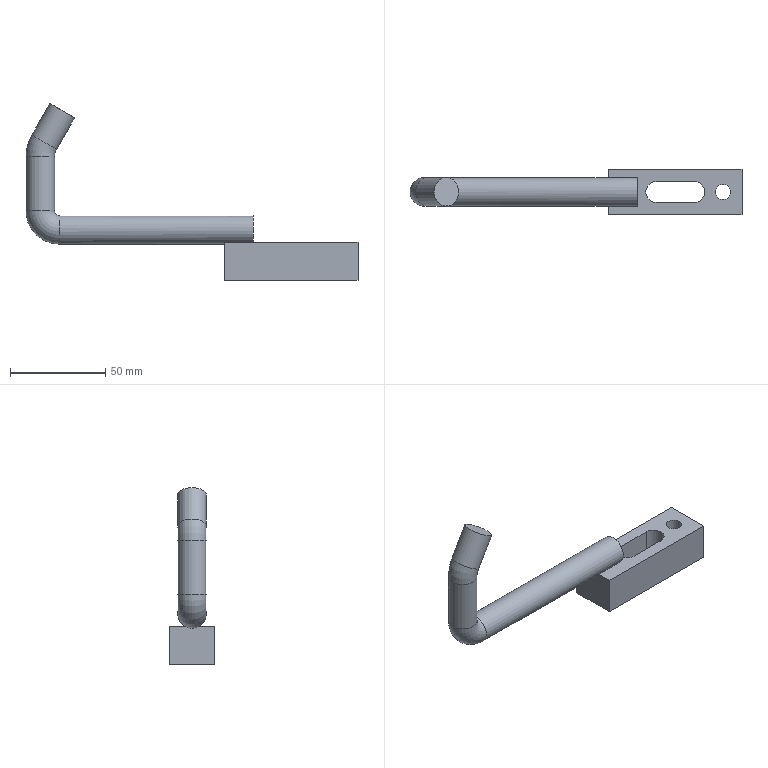Part | NX | features solid 2 | 1 solid | 18 faces | box 174.2 x 24 x 92.75 mm | volume 56758 mm3 | plane 10 | cylinder 6 | torus 2 | commonest cylinder face diameters 15 x3 11 x2 8 x1
STEP:
#1=CARTESIAN_POINT('',(-380.,96.04,-15.));
#2=VERTEX_POINT('',#1);
#3=CARTESIAN_POINT('',(-380.,120.04,-15.));
#4=VERTEX_POINT('',#3);
#5=CARTESIAN_POINT('',(-380.,96.04,-15.));
#6=DIRECTION('',(0.,1.,0.));
#7=VECTOR('',#6,1000.);
#8=LINE('',#5,#7);
#9=EDGE_CURVE('',#2,#4,#8,.T.);
#10=ORIENTED_EDGE('',*,*,#9,.T.);
#11=CARTESIAN_POINT('',(-310.,120.04,-15.));
#12=VERTEX_POINT('',#11);
#13=CARTESIAN_POINT('',(-380.,120.04,-15.));
#14=DIRECTION('',(1.,0.,0.));
#15=VECTOR('',#14,1000.);
#16=LINE('',#13,#15);
#17=EDGE_CURVE('',#4,#12,#16,.T.);
#18=ORIENTED_EDGE('',*,*,#17,.T.);
#19=CARTESIAN_POINT('',(-310.,96.04,-15.));
#20=VERTEX_POINT('',#19);
#21=CARTESIAN_POINT('',(-310.,120.04,-15.));
#22=DIRECTION('',(0.,-1.,0.));
#23=VECTOR('',#22,1000.);
#24=LINE('',#21,#23);
#25=EDGE_CURVE('',#12,#20,#24,.T.);
#26=ORIENTED_EDGE('',*,*,#25,.T.);
#27=CARTESIAN_POINT('',(-310.,96.04,-15.));
#28=DIRECTION('',(-1.,0.,0.));
#29=VECTOR('',#28,1000.);
#30=LINE('',#27,#29);
#31=EDGE_CURVE('',#20,#2,#30,.T.);
#32=ORIENTED_EDGE('',*,*,#31,.T.);
#33=EDGE_LOOP('',(#10,#18,#26,#32));
#34=FACE_BOUND('',#33,.T.);
#35=CARTESIAN_POINT('',(-335.,113.54,-15.));
#36=VERTEX_POINT('',#35);
#37=CARTESIAN_POINT('',(-335.,102.54,-15.));
#38=VERTEX_POINT('',#37);
#39=CARTESIAN_POINT('',(-335.,108.04,-15.));
#40=DIRECTION('',(0.,0.,-1.));
#41=DIRECTION('',(1.,0.,0.));
#42=AXIS2_PLACEMENT_3D('',#39,#40,#41);
#43=CIRCLE('',#42,5.5);
#44=EDGE_CURVE('',#36,#38,#43,.T.);
#45=ORIENTED_EDGE('',*,*,#44,.F.);
#46=CARTESIAN_POINT('',(-355.,113.54,-15.));
#47=VERTEX_POINT('',#46);
#48=CARTESIAN_POINT('',(-355.,113.54,-15.));
#49=DIRECTION('',(1.,0.,0.));
#50=VECTOR('',#49,1000.);
#51=LINE('',#48,#50);
#52=EDGE_CURVE('',#47,#36,#51,.T.);
#53=ORIENTED_EDGE('',*,*,#52,.F.);
#54=CARTESIAN_POINT('',(-355.,102.54,-15.));
#55=VERTEX_POINT('',#54);
#56=CARTESIAN_POINT('',(-355.,108.04,-15.));
#57=DIRECTION('',(0.,0.,-1.));
#58=DIRECTION('',(1.,0.,0.));
#59=AXIS2_PLACEMENT_3D('',#56,#57,#58);
#60=CIRCLE('',#59,5.5);
#61=EDGE_CURVE('',#55,#47,#60,.T.);
#62=ORIENTED_EDGE('',*,*,#61,.F.);
#63=CARTESIAN_POINT('',(-355.,102.54,-15.));
#64=DIRECTION('',(1.,0.,0.));
#65=VECTOR('',#64,1000.);
#66=LINE('',#63,#65);
#67=EDGE_CURVE('',#55,#38,#66,.T.);
#68=ORIENTED_EDGE('',*,*,#67,.T.);
#69=EDGE_LOOP('',(#45,#53,#62,#68));
#70=FACE_BOUND('',#69,.T.);
#71=CARTESIAN_POINT('',(-316.,108.04,-15.));
#72=VERTEX_POINT('',#71);
#73=CARTESIAN_POINT('',(-320.,108.04,-15.));
#74=DIRECTION('',(0.,0.,-1.));
#75=DIRECTION('',(1.,0.,0.));
#76=AXIS2_PLACEMENT_3D('',#73,#74,#75);
#77=CIRCLE('',#76,4.);
#78=EDGE_CURVE('',#72,#72,#77,.T.);
#79=ORIENTED_EDGE('',*,*,#78,.F.);
#80=EDGE_LOOP('',(#79));
#81=FACE_BOUND('',#80,.T.);
#82=CARTESIAN_POINT('',(-310.,96.04,-15.));
#83=DIRECTION('',(0.,0.,1.));
#84=DIRECTION('',(1.,0.,0.));
#85=AXIS2_PLACEMENT_3D('',#82,#83,#84);
#86=PLANE('',#85);
#87=ADVANCED_FACE('',(#34,#70,#81),#86,.F.);
#88=ORIENTED_EDGE('',*,*,#17,.F.);
#89=CARTESIAN_POINT('',(-380.,120.04,5.));
#90=VERTEX_POINT('',#89);
#91=CARTESIAN_POINT('',(-380.,120.04,5.));
#92=DIRECTION('',(0.,0.,-1.));
#93=VECTOR('',#92,1000.);
#94=LINE('',#91,#93);
#95=EDGE_CURVE('',#90,#4,#94,.T.);
#96=ORIENTED_EDGE('',*,*,#95,.F.);
#97=CARTESIAN_POINT('',(-310.,120.04,5.));
#98=VERTEX_POINT('',#97);
#99=CARTESIAN_POINT('',(-380.,120.04,5.));
#100=DIRECTION('',(1.,0.,0.));
#101=VECTOR('',#100,1000.);
#102=LINE('',#99,#101);
#103=EDGE_CURVE('',#90,#98,#102,.T.);
#104=ORIENTED_EDGE('',*,*,#103,.T.);
#105=CARTESIAN_POINT('',(-310.,120.04,5.));
#106=DIRECTION('',(0.,0.,-1.));
#107=VECTOR('',#106,1000.);
#108=LINE('',#105,#107);
#109=EDGE_CURVE('',#98,#12,#108,.T.);
#110=ORIENTED_EDGE('',*,*,#109,.T.);
#111=EDGE_LOOP('',(#88,#96,#104,#110));
#112=FACE_BOUND('',#111,.T.);
#113=CARTESIAN_POINT('',(-380.,120.04,5.));
#114=DIRECTION('',(0.,-1.,0.));
#115=DIRECTION('',(-1.,0.,0.));
#116=AXIS2_PLACEMENT_3D('',#113,#114,#115);
#117=PLANE('',#116);
#118=ADVANCED_FACE('',(#112),#117,.F.);
#119=ORIENTED_EDGE('',*,*,#25,.F.);
#120=ORIENTED_EDGE('',*,*,#109,.F.);
#121=CARTESIAN_POINT('',(-310.,96.04,5.));
#122=VERTEX_POINT('',#121);
#123=CARTESIAN_POINT('',(-310.,120.04,5.));
#124=DIRECTION('',(0.,-1.,0.));
#125=VECTOR('',#124,1000.);
#126=LINE('',#123,#125);
#127=EDGE_CURVE('',#98,#122,#126,.T.);
#128=ORIENTED_EDGE('',*,*,#127,.T.);
#129=CARTESIAN_POINT('',(-310.,96.04,5.));
#130=DIRECTION('',(0.,0.,-1.));
#131=VECTOR('',#130,1000.);
#132=LINE('',#129,#131);
#133=EDGE_CURVE('',#122,#20,#132,.T.);
#134=ORIENTED_EDGE('',*,*,#133,.T.);
#135=EDGE_LOOP('',(#119,#120,#128,#134));
#136=FACE_BOUND('',#135,.T.);
#137=CARTESIAN_POINT('',(-310.,120.04,5.));
#138=DIRECTION('',(-1.,0.,0.));
#139=DIRECTION('',(0.,0.,1.));
#140=AXIS2_PLACEMENT_3D('',#137,#138,#139);
#141=PLANE('',#140);
#142=ADVANCED_FACE('',(#136),#141,.F.);
#143=ORIENTED_EDGE('',*,*,#31,.F.);
#144=ORIENTED_EDGE('',*,*,#133,.F.);
#145=CARTESIAN_POINT('',(-380.,96.04,5.));
#146=VERTEX_POINT('',#145);
#147=CARTESIAN_POINT('',(-310.,96.04,5.));
#148=DIRECTION('',(-1.,0.,0.));
#149=VECTOR('',#148,1000.);
#150=LINE('',#147,#149);
#151=EDGE_CURVE('',#122,#146,#150,.T.);
#152=ORIENTED_EDGE('',*,*,#151,.T.);
#153=CARTESIAN_POINT('',(-380.,96.04,5.));
#154=DIRECTION('',(0.,0.,-1.));
#155=VECTOR('',#154,1000.);
#156=LINE('',#153,#155);
#157=EDGE_CURVE('',#146,#2,#156,.T.);
#158=ORIENTED_EDGE('',*,*,#157,.T.);
#159=EDGE_LOOP('',(#143,#144,#152,#158));
#160=FACE_BOUND('',#159,.T.);
#161=CARTESIAN_POINT('',(-310.,96.04,5.));
#162=DIRECTION('',(0.,1.,0.));
#163=DIRECTION('',(1.,0.,0.));
#164=AXIS2_PLACEMENT_3D('',#161,#162,#163);
#165=PLANE('',#164);
#166=ADVANCED_FACE('',(#160),#165,.F.);
#167=CARTESIAN_POINT('',(-380.,104.298,5.));
#168=VERTEX_POINT('',#167);
#169=CARTESIAN_POINT('',(-380.,96.04,5.));
#170=DIRECTION('',(0.,1.,0.));
#171=VECTOR('',#170,1000.);
#172=LINE('',#169,#171);
#173=EDGE_CURVE('',#146,#168,#172,.T.);
#174=ORIENTED_EDGE('',*,*,#173,.T.);
#175=CARTESIAN_POINT('',(-380.,111.781,5.));
#176=VERTEX_POINT('',#175);
#177=CARTESIAN_POINT('',(-380.,108.04,11.5));
#178=DIRECTION('',(1.,0.,0.));
#179=DIRECTION('',(0.,0.,-1.));
#180=AXIS2_PLACEMENT_3D('',#177,#178,#179);
#181=CIRCLE('',#180,7.5);
#182=EDGE_CURVE('',#168,#176,#181,.T.);
#183=ORIENTED_EDGE('',*,*,#182,.T.);
#184=CARTESIAN_POINT('',(-380.,96.04,5.));
#185=DIRECTION('',(0.,1.,0.));
#186=VECTOR('',#185,1000.);
#187=LINE('',#184,#186);
#188=EDGE_CURVE('',#176,#90,#187,.T.);
#189=ORIENTED_EDGE('',*,*,#188,.T.);
#190=ORIENTED_EDGE('',*,*,#95,.T.);
#191=ORIENTED_EDGE('',*,*,#9,.F.);
#192=ORIENTED_EDGE('',*,*,#157,.F.);
#193=EDGE_LOOP('',(#174,#183,#189,#190,#191,#192));
#194=FACE_BOUND('',#193,.T.);
#195=CARTESIAN_POINT('',(-380.,96.04,5.));
#196=DIRECTION('',(1.,0.,0.));
#197=DIRECTION('',(0.,0.,-1.));
#198=AXIS2_PLACEMENT_3D('',#195,#196,#197);
#199=PLANE('',#198);
#200=ADVANCED_FACE('',(#194),#199,.F.);
#201=CARTESIAN_POINT('',(-335.,113.54,5.));
#202=VERTEX_POINT('',#201);
#203=CARTESIAN_POINT('',(-335.,102.54,5.));
#204=VERTEX_POINT('',#203);
#205=CARTESIAN_POINT('',(-335.,108.04,5.));
#206=DIRECTION('',(0.,0.,-1.));
#207=DIRECTION('',(1.,0.,0.));
#208=AXIS2_PLACEMENT_3D('',#205,#206,#207);
#209=CIRCLE('',#208,5.5);
#210=EDGE_CURVE('',#202,#204,#209,.T.);
#211=ORIENTED_EDGE('',*,*,#210,.F.);
#212=CARTESIAN_POINT('',(-335.,113.54,5.));
#213=DIRECTION('',(0.,0.,1.));
#214=VECTOR('',#213,1000.);
#215=LINE('',#212,#214);
#216=EDGE_CURVE('',#36,#202,#215,.T.);
#217=ORIENTED_EDGE('',*,*,#216,.F.);
#218=ORIENTED_EDGE('',*,*,#44,.T.);
#219=CARTESIAN_POINT('',(-335.,102.54,5.));
#220=DIRECTION('',(0.,0.,1.));
#221=VECTOR('',#220,1000.);
#222=LINE('',#219,#221);
#223=EDGE_CURVE('',#38,#204,#222,.T.);
#224=ORIENTED_EDGE('',*,*,#223,.T.);
#225=EDGE_LOOP('',(#211,#217,#218,#224));
#226=FACE_BOUND('',#225,.T.);
#227=CARTESIAN_POINT('',(-335.,108.04,5.));
#228=DIRECTION('',(0.,0.,1.));
#229=DIRECTION('',(1.,0.,0.));
#230=AXIS2_PLACEMENT_3D('',#227,#228,#229);
#231=CYLINDRICAL_SURFACE('',#230,5.5);
#232=ADVANCED_FACE('',(#226),#231,.F.);
#233=CARTESIAN_POINT('',(-355.,113.54,5.));
#234=VERTEX_POINT('',#233);
#235=CARTESIAN_POINT('',(-345.,113.54,5.));
#236=DIRECTION('',(1.,0.,0.));
#237=VECTOR('',#236,1000.);
#238=LINE('',#235,#237);
#239=EDGE_CURVE('',#234,#202,#238,.T.);
#240=ORIENTED_EDGE('',*,*,#239,.F.);
#241=CARTESIAN_POINT('',(-355.,113.54,5.));
#242=DIRECTION('',(0.,0.,1.));
#243=VECTOR('',#242,1000.);
#244=LINE('',#241,#243);
#245=EDGE_CURVE('',#47,#234,#244,.T.);
#246=ORIENTED_EDGE('',*,*,#245,.F.);
#247=ORIENTED_EDGE('',*,*,#52,.T.);
#248=ORIENTED_EDGE('',*,*,#216,.T.);
#249=EDGE_LOOP('',(#240,#246,#247,#248));
#250=FACE_BOUND('',#249,.T.);
#251=CARTESIAN_POINT('',(-345.,113.54,5.));
#252=DIRECTION('',(0.,1.,0.));
#253=DIRECTION('',(0.,0.,-1.));
#254=AXIS2_PLACEMENT_3D('',#251,#252,#253);
#255=PLANE('',#254);
#256=ADVANCED_FACE('',(#250),#255,.F.);
#257=CARTESIAN_POINT('',(-355.,102.54,5.));
#258=VERTEX_POINT('',#257);
#259=CARTESIAN_POINT('',(-355.,108.04,5.));
#260=DIRECTION('',(0.,0.,-1.));
#261=DIRECTION('',(1.,0.,0.));
#262=AXIS2_PLACEMENT_3D('',#259,#260,#261);
#263=CIRCLE('',#262,5.5);
#264=EDGE_CURVE('',#258,#234,#263,.T.);
#265=ORIENTED_EDGE('',*,*,#264,.F.);
#266=CARTESIAN_POINT('',(-355.,102.54,5.));
#267=DIRECTION('',(0.,0.,1.));
#268=VECTOR('',#267,1000.);
#269=LINE('',#266,#268);
#270=EDGE_CURVE('',#55,#258,#269,.T.);
#271=ORIENTED_EDGE('',*,*,#270,.F.);
#272=ORIENTED_EDGE('',*,*,#61,.T.);
#273=ORIENTED_EDGE('',*,*,#245,.T.);
#274=EDGE_LOOP('',(#265,#271,#272,#273));
#275=FACE_BOUND('',#274,.T.);
#276=CARTESIAN_POINT('',(-355.,108.04,5.));
#277=DIRECTION('',(0.,0.,1.));
#278=DIRECTION('',(1.,0.,0.));
#279=AXIS2_PLACEMENT_3D('',#276,#277,#278);
#280=CYLINDRICAL_SURFACE('',#279,5.5);
#281=ADVANCED_FACE('',(#275),#280,.F.);
#282=CARTESIAN_POINT('',(-345.,102.54,5.));
#283=DIRECTION('',(1.,0.,0.));
#284=VECTOR('',#283,1000.);
#285=LINE('',#282,#284);
#286=EDGE_CURVE('',#258,#204,#285,.T.);
#287=ORIENTED_EDGE('',*,*,#286,.T.);
#288=ORIENTED_EDGE('',*,*,#223,.F.);
#289=ORIENTED_EDGE('',*,*,#67,.F.);
#290=ORIENTED_EDGE('',*,*,#270,.T.);
#291=EDGE_LOOP('',(#287,#288,#289,#290));
#292=FACE_BOUND('',#291,.T.);
#293=CARTESIAN_POINT('',(-345.,102.54,5.));
#294=DIRECTION('',(0.,-1.,0.));
#295=DIRECTION('',(0.,0.,1.));
#296=AXIS2_PLACEMENT_3D('',#293,#294,#295);
#297=PLANE('',#296);
#298=ADVANCED_FACE('',(#292),#297,.F.);
#299=CARTESIAN_POINT('',(-324.,108.04,5.));
#300=VERTEX_POINT('',#299);
#301=CARTESIAN_POINT('',(-320.,108.04,5.));
#302=DIRECTION('',(0.,0.,1.));
#303=DIRECTION('',(-1.,0.,0.));
#304=AXIS2_PLACEMENT_3D('',#301,#302,#303);
#305=CIRCLE('',#304,4.);
#306=EDGE_CURVE('',#300,#300,#305,.T.);
#307=ORIENTED_EDGE('',*,*,#306,.T.);
#308=EDGE_LOOP('',(#307));
#309=FACE_BOUND('',#308,.T.);
#310=ORIENTED_EDGE('',*,*,#78,.T.);
#311=EDGE_LOOP('',(#310));
#312=FACE_BOUND('',#311,.T.);
#313=CARTESIAN_POINT('',(-320.,108.04,5.));
#314=DIRECTION('',(0.,0.,-1.));
#315=DIRECTION('',(-1.,0.,0.));
#316=AXIS2_PLACEMENT_3D('',#313,#314,#315);
#317=CYLINDRICAL_SURFACE('',#316,4.);
#318=ADVANCED_FACE('',(#309,#312),#317,.F.);
#319=CARTESIAN_POINT('',(-365.,104.298,5.));
#320=VERTEX_POINT('',#319);
#321=CARTESIAN_POINT('',(-466.7,104.298,5.));
#322=DIRECTION('',(1.,0.,0.));
#323=VECTOR('',#322,1000.);
#324=LINE('',#321,#323);
#325=EDGE_CURVE('',#168,#320,#324,.T.);
#326=ORIENTED_EDGE('',*,*,#325,.F.);
#327=ORIENTED_EDGE('',*,*,#173,.F.);
#328=ORIENTED_EDGE('',*,*,#151,.F.);
#329=ORIENTED_EDGE('',*,*,#127,.F.);
#330=ORIENTED_EDGE('',*,*,#103,.F.);
#331=ORIENTED_EDGE('',*,*,#188,.F.);
#332=CARTESIAN_POINT('',(-365.,111.781,5.));
#333=VERTEX_POINT('',#332);
#334=CARTESIAN_POINT('',(-466.7,111.781,5.));
#335=DIRECTION('',(1.,0.,0.));
#336=VECTOR('',#335,1000.);
#337=LINE('',#334,#336);
#338=EDGE_CURVE('',#333,#176,#337,.F.);
#339=ORIENTED_EDGE('',*,*,#338,.F.);
#340=CARTESIAN_POINT('',(-365.,96.04,5.));
#341=DIRECTION('',(0.,1.,0.));
#342=VECTOR('',#341,1000.);
#343=LINE('',#340,#342);
#344=EDGE_CURVE('',#320,#333,#343,.T.);
#345=ORIENTED_EDGE('',*,*,#344,.F.);
#346=EDGE_LOOP('',(#326,#327,#328,#329,#330,#331,#339,#345));
#347=FACE_BOUND('',#346,.T.);
#348=ORIENTED_EDGE('',*,*,#306,.F.);
#349=EDGE_LOOP('',(#348));
#350=FACE_BOUND('',#349,.T.);
#351=ORIENTED_EDGE('',*,*,#286,.F.);
#352=ORIENTED_EDGE('',*,*,#264,.T.);
#353=ORIENTED_EDGE('',*,*,#239,.T.);
#354=ORIENTED_EDGE('',*,*,#210,.T.);
#355=EDGE_LOOP('',(#351,#352,#353,#354));
#356=FACE_BOUND('',#355,.T.);
#357=CARTESIAN_POINT('',(-310.,96.04,5.));
#358=DIRECTION('',(0.,0.,1.));
#359=DIRECTION('',(1.,0.,0.));
#360=AXIS2_PLACEMENT_3D('',#357,#358,#359);
#361=PLANE('',#360);
#362=ADVANCED_FACE('',(#347,#350,#356),#361,.T.);
#363=CARTESIAN_POINT('',(-469.2,108.04,49.981));
#364=VERTEX_POINT('',#363);
#365=CARTESIAN_POINT('',(-476.7,108.04,49.981));
#366=DIRECTION('',(0.,0.,-1.));
#367=DIRECTION('',(1.,0.,0.));
#368=AXIS2_PLACEMENT_3D('',#365,#366,#367);
#369=CIRCLE('',#368,7.5);
#370=EDGE_CURVE('',#364,#364,#369,.T.);
#371=ORIENTED_EDGE('',*,*,#370,.T.);
#372=EDGE_LOOP('',(#371));
#373=FACE_BOUND('',#372,.T.);
#374=CARTESIAN_POINT('',(-484.2,108.04,21.5));
#375=VERTEX_POINT('',#374);
#376=CARTESIAN_POINT('',(-476.7,108.04,21.5));
#377=DIRECTION('',(0.,0.,-1.));
#378=DIRECTION('',(-1.,0.,0.));
#379=AXIS2_PLACEMENT_3D('',#376,#377,#378);
#380=CIRCLE('',#379,7.5);
#381=EDGE_CURVE('',#375,#375,#380,.T.);
#382=ORIENTED_EDGE('',*,*,#381,.F.);
#383=EDGE_LOOP('',(#382));
#384=FACE_BOUND('',#383,.T.);
#385=CARTESIAN_POINT('',(-476.7,108.04,-40.019));
#386=DIRECTION('',(0.,0.,-1.));
#387=DIRECTION('',(-1.,0.,0.));
#388=AXIS2_PLACEMENT_3D('',#385,#386,#387);
#389=CYLINDRICAL_SURFACE('',#388,7.5);
#390=ADVANCED_FACE('',(#373,#384),#389,.T.);
#391=CARTESIAN_POINT('',(-468.195,108.04,53.731));
#392=VERTEX_POINT('',#391);
#393=CARTESIAN_POINT('',(-474.69,108.04,57.481));
#394=DIRECTION('',(-0.5,0.,-0.866));
#395=DIRECTION('',(0.866,0.,-0.5));
#396=AXIS2_PLACEMENT_3D('',#393,#394,#395);
#397=CIRCLE('',#396,7.5);
#398=EDGE_CURVE('',#392,#392,#397,.T.);
#399=ORIENTED_EDGE('',*,*,#398,.F.);
#400=EDGE_LOOP('',(#399));
#401=FACE_BOUND('',#400,.T.);
#402=CARTESIAN_POINT('',(-458.658,108.04,70.25));
#403=VERTEX_POINT('',#402);
#404=CARTESIAN_POINT('',(-465.153,108.04,74.));
#405=DIRECTION('',(-0.5,0.,-0.866));
#406=DIRECTION('',(0.866,0.,-0.5));
#407=AXIS2_PLACEMENT_3D('',#404,#405,#406);
#408=CIRCLE('',#407,7.5);
#409=EDGE_CURVE('',#403,#403,#408,.T.);
#410=ORIENTED_EDGE('',*,*,#409,.T.);
#411=EDGE_LOOP('',(#410));
#412=FACE_BOUND('',#411,.T.);
#413=CARTESIAN_POINT('',(-474.69,108.04,57.481));
#414=DIRECTION('',(0.5,0.,0.866));
#415=DIRECTION('',(0.866,0.,-0.5));
#416=AXIS2_PLACEMENT_3D('',#413,#414,#415);
#417=CYLINDRICAL_SURFACE('',#416,7.5);
#418=ADVANCED_FACE('',(#401,#412),#417,.T.);
#419=ORIENTED_EDGE('',*,*,#370,.F.);
#420=EDGE_LOOP('',(#419));
#421=FACE_BOUND('',#420,.T.);
#422=ORIENTED_EDGE('',*,*,#398,.T.);
#423=EDGE_LOOP('',(#422));
#424=FACE_BOUND('',#423,.T.);
#425=CARTESIAN_POINT('',(-461.7,108.04,49.981));
#426=DIRECTION('',(0.,-1.,0.));
#427=DIRECTION('',(0.,0.,1.));
#428=AXIS2_PLACEMENT_3D('',#425,#426,#427);
#429=TOROIDAL_SURFACE('',#428,15.,7.5);
#430=ADVANCED_FACE('',(#421,#424),#429,.T.);
#431=ORIENTED_EDGE('',*,*,#409,.F.);
#432=EDGE_LOOP('',(#431));
#433=FACE_BOUND('',#432,.T.);
#434=CARTESIAN_POINT('',(-465.153,108.04,74.));
#435=DIRECTION('',(0.5,0.,0.866));
#436=DIRECTION('',(0.866,0.,-0.5));
#437=AXIS2_PLACEMENT_3D('',#434,#435,#436);
#438=PLANE('',#437);
#439=ADVANCED_FACE('',(#433),#438,.T.);
#440=CARTESIAN_POINT('',(-466.7,108.04,4.));
#441=VERTEX_POINT('',#440);
#442=CARTESIAN_POINT('',(-466.7,108.04,11.5));
#443=DIRECTION('',(1.,0.,0.));
#444=DIRECTION('',(0.,0.,-1.));
#445=AXIS2_PLACEMENT_3D('',#442,#443,#444);
#446=CIRCLE('',#445,7.5);
#447=EDGE_CURVE('',#441,#441,#446,.T.);
#448=ORIENTED_EDGE('',*,*,#447,.F.);
#449=EDGE_LOOP('',(#448));
#450=FACE_BOUND('',#449,.T.);
#451=ORIENTED_EDGE('',*,*,#381,.T.);
#452=EDGE_LOOP('',(#451));
#453=FACE_BOUND('',#452,.T.);
#454=CARTESIAN_POINT('',(-466.7,108.04,21.5));
#455=DIRECTION('',(0.,1.,0.));
#456=DIRECTION('',(0.,0.,1.));
#457=AXIS2_PLACEMENT_3D('',#454,#455,#456);
#458=TOROIDAL_SURFACE('',#457,10.,7.5);
#459=ADVANCED_FACE('',(#450,#453),#458,.T.);
#460=ORIENTED_EDGE('',*,*,#447,.T.);
#461=EDGE_LOOP('',(#460));
#462=FACE_BOUND('',#461,.T.);
#463=ORIENTED_EDGE('',*,*,#182,.F.);
#464=ORIENTED_EDGE('',*,*,#325,.T.);
#465=CARTESIAN_POINT('',(-365.,108.04,11.5));
#466=DIRECTION('',(1.,0.,0.));
#467=DIRECTION('',(0.,0.,-1.));
#468=AXIS2_PLACEMENT_3D('',#465,#466,#467);
#469=CIRCLE('',#468,7.5);
#470=EDGE_CURVE('',#333,#320,#469,.T.);
#471=ORIENTED_EDGE('',*,*,#470,.F.);
#472=ORIENTED_EDGE('',*,*,#338,.T.);
#473=EDGE_LOOP('',(#463,#464,#471,#472));
#474=FACE_BOUND('',#473,.T.);
#475=CARTESIAN_POINT('',(-466.7,108.04,11.5));
#476=DIRECTION('',(1.,0.,0.));
#477=DIRECTION('',(0.,0.,-1.));
#478=AXIS2_PLACEMENT_3D('',#475,#476,#477);
#479=CYLINDRICAL_SURFACE('',#478,7.5);
#480=ADVANCED_FACE('',(#462,#474),#479,.T.);
#481=ORIENTED_EDGE('',*,*,#470,.T.);
#482=ORIENTED_EDGE('',*,*,#344,.T.);
#483=EDGE_LOOP('',(#481,#482));
#484=FACE_BOUND('',#483,.T.);
#485=CARTESIAN_POINT('',(-365.,108.04,11.5));
#486=DIRECTION('',(1.,0.,0.));
#487=DIRECTION('',(0.,0.,-1.));
#488=AXIS2_PLACEMENT_3D('',#485,#486,#487);
#489=PLANE('',#488);
#490=ADVANCED_FACE('',(#484),#489,.T.);
#491=CLOSED_SHELL('',(#87,#118,#142,#166,#200,#232,#256,#281,#298,#318,#362,#390,#418,#430,#439,#459,#480,#490));
#492=MANIFOLD_SOLID_BREP('',#491);
#493=(LENGTH_UNIT()NAMED_UNIT(*)SI_UNIT(.MILLI.,.METRE.));
#494=UNCERTAINTY_MEASURE_WITH_UNIT(LENGTH_MEASURE(0.00001),#493,'','');
#495=(NAMED_UNIT(*)PLANE_ANGLE_UNIT()SI_UNIT($,.RADIAN.));
#496=(NAMED_UNIT(*)SI_UNIT($,.STERADIAN.)SOLID_ANGLE_UNIT());
#497=(GEOMETRIC_REPRESENTATION_CONTEXT(3)GLOBAL_UNCERTAINTY_ASSIGNED_CONTEXT((#494))GLOBAL_UNIT_ASSIGNED_CONTEXT((#493,#495,#496))REPRESENTATION_CONTEXT('',''));
#498=ADVANCED_BREP_SHAPE_REPRESENTATION('',(#492),#497);